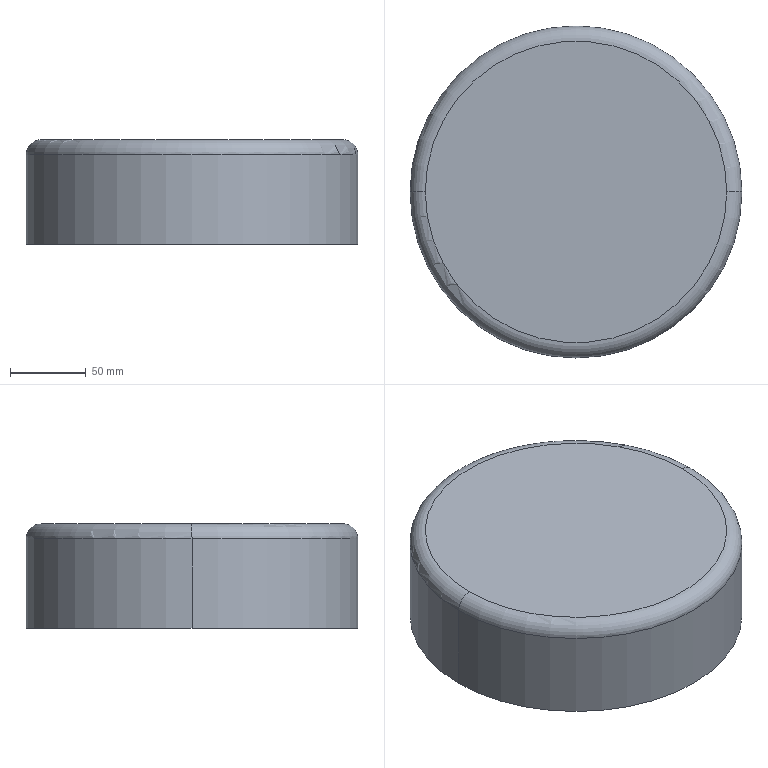Part | SolidWorks | features Fillet 2, Extrusion 1, Shell 1 | 1 solid | 11 faces | box 219 x 219 x 69 mm | volume 466703 mm3 | torus 4 | cylinder 4 | plane 3 | commonest cylinder face diameters 207 x2 219 x2
STEP:
#1=CARTESIAN_POINT('',(-103.5,0.,59.));
#2=VERTEX_POINT('',#1);
#3=CARTESIAN_POINT('',(103.5,0.,59.));
#4=VERTEX_POINT('',#3);
#5=CARTESIAN_POINT('',(0.,0.,59.));
#6=DIRECTION('',(0.,0.,1.));
#7=DIRECTION('',(1.,0.,0.));
#8=AXIS2_PLACEMENT_3D('',#5,#6,#7);
#9=CIRCLE('',#8,103.5);
#10=EDGE_CURVE('',#2,#4,#9,.T.);
#11=ORIENTED_EDGE('',*,*,#10,.F.);
#12=CARTESIAN_POINT('',(-99.5,0.,63.));
#13=VERTEX_POINT('',#12);
#14=CARTESIAN_POINT('',(-99.5,0.,59.));
#15=DIRECTION('',(0.,1.,0.));
#16=DIRECTION('',(-1.,0.,0.));
#17=AXIS2_PLACEMENT_3D('',#14,#15,#16);
#18=CIRCLE('',#17,4.);
#19=EDGE_CURVE('',#2,#13,#18,.T.);
#20=ORIENTED_EDGE('',*,*,#19,.T.);
#21=CARTESIAN_POINT('',(99.5,0.,63.));
#22=VERTEX_POINT('',#21);
#23=CARTESIAN_POINT('',(0.,0.,63.));
#24=DIRECTION('',(0.,0.,-1.));
#25=DIRECTION('',(1.,0.,0.));
#26=AXIS2_PLACEMENT_3D('',#23,#24,#25);
#27=CIRCLE('',#26,99.5);
#28=EDGE_CURVE('',#22,#13,#27,.T.);
#29=ORIENTED_EDGE('',*,*,#28,.F.);
#30=CARTESIAN_POINT('',(99.5,0.,59.));
#31=DIRECTION('',(0.,-1.,0.));
#32=DIRECTION('',(0.,0.,-1.));
#33=AXIS2_PLACEMENT_3D('',#30,#31,#32);
#34=CIRCLE('',#33,4.);
#35=EDGE_CURVE('',#4,#22,#34,.T.);
#36=ORIENTED_EDGE('',*,*,#35,.F.);
#37=EDGE_LOOP('',(#11,#20,#29,#36));
#38=FACE_OUTER_BOUND('',#37,.T.);
#39=CARTESIAN_POINT('',(0.,0.,59.));
#40=DIRECTION('',(0.,0.,1.));
#41=DIRECTION('',(1.,0.,0.));
#42=AXIS2_PLACEMENT_3D('',#39,#40,#41);
#43=TOROIDAL_SURFACE('',#42,99.5,4.);
#44=ADVANCED_FACE('',(#38),#43,.F.);
#45=CARTESIAN_POINT('',(-109.5,0.,59.));
#46=VERTEX_POINT('',#45);
#47=CARTESIAN_POINT('',(109.5,0.,59.));
#48=VERTEX_POINT('',#47);
#49=CARTESIAN_POINT('',(0.,0.,59.));
#50=DIRECTION('',(0.,0.,-1.));
#51=DIRECTION('',(1.,0.,0.));
#52=AXIS2_PLACEMENT_3D('',#49,#50,#51);
#53=CIRCLE('',#52,109.5);
#54=EDGE_CURVE('',#46,#48,#53,.T.);
#55=ORIENTED_EDGE('',*,*,#54,.F.);
#56=CARTESIAN_POINT('',(-99.5,0.,69.));
#57=VERTEX_POINT('',#56);
#58=CARTESIAN_POINT('',(-99.5,0.,59.));
#59=DIRECTION('',(0.,1.,0.));
#60=DIRECTION('',(-1.,0.,0.));
#61=AXIS2_PLACEMENT_3D('',#58,#59,#60);
#62=CIRCLE('',#61,10.);
#63=EDGE_CURVE('',#46,#57,#62,.T.);
#64=ORIENTED_EDGE('',*,*,#63,.T.);
#65=CARTESIAN_POINT('',(99.5,0.,69.));
#66=VERTEX_POINT('',#65);
#67=CARTESIAN_POINT('',(0.,0.,69.));
#68=DIRECTION('',(0.,0.,1.));
#69=DIRECTION('',(1.,0.,0.));
#70=AXIS2_PLACEMENT_3D('',#67,#68,#69);
#71=CIRCLE('',#70,99.5);
#72=EDGE_CURVE('',#66,#57,#71,.T.);
#73=ORIENTED_EDGE('',*,*,#72,.F.);
#74=CARTESIAN_POINT('',(99.5,0.,59.));
#75=DIRECTION('',(0.,-1.,0.));
#76=DIRECTION('',(0.,0.,-1.));
#77=AXIS2_PLACEMENT_3D('',#74,#75,#76);
#78=CIRCLE('',#77,10.);
#79=EDGE_CURVE('',#48,#66,#78,.T.);
#80=ORIENTED_EDGE('',*,*,#79,.F.);
#81=EDGE_LOOP('',(#55,#64,#73,#80));
#82=FACE_OUTER_BOUND('',#81,.T.);
#83=CARTESIAN_POINT('',(0.,0.,59.));
#84=DIRECTION('',(0.,0.,1.));
#85=DIRECTION('',(1.,0.,0.));
#86=AXIS2_PLACEMENT_3D('',#83,#84,#85);
#87=TOROIDAL_SURFACE('',#86,99.5,10.);
#88=ADVANCED_FACE('',(#82),#87,.T.);
#89=ORIENTED_EDGE('',*,*,#10,.T.);
#90=CARTESIAN_POINT('',(103.5,0.,0.));
#91=VERTEX_POINT('',#90);
#92=CARTESIAN_POINT('',(103.5,0.,69.));
#93=DIRECTION('',(0.,0.,-1.));
#94=VECTOR('',#93,1000.);
#95=LINE('',#92,#94);
#96=EDGE_CURVE('',#4,#91,#95,.T.);
#97=ORIENTED_EDGE('',*,*,#96,.T.);
#98=CARTESIAN_POINT('',(-103.5,0.,0.));
#99=VERTEX_POINT('',#98);
#100=CARTESIAN_POINT('',(0.,0.,0.));
#101=DIRECTION('',(0.,0.,1.));
#102=DIRECTION('',(1.,0.,0.));
#103=AXIS2_PLACEMENT_3D('',#100,#101,#102);
#104=CIRCLE('',#103,103.5);
#105=EDGE_CURVE('',#99,#91,#104,.T.);
#106=ORIENTED_EDGE('',*,*,#105,.F.);
#107=CARTESIAN_POINT('',(-103.5,0.,69.));
#108=DIRECTION('',(0.,0.,-1.));
#109=VECTOR('',#108,1000.);
#110=LINE('',#107,#109);
#111=EDGE_CURVE('',#2,#99,#110,.T.);
#112=ORIENTED_EDGE('',*,*,#111,.F.);
#113=EDGE_LOOP('',(#89,#97,#106,#112));
#114=FACE_OUTER_BOUND('',#113,.T.);
#115=CARTESIAN_POINT('',(0.,0.,69.));
#116=DIRECTION('',(0.,0.,-1.));
#117=DIRECTION('',(-1.,0.,0.));
#118=AXIS2_PLACEMENT_3D('',#115,#116,#117);
#119=CYLINDRICAL_SURFACE('',#118,103.5);
#120=ADVANCED_FACE('',(#114),#119,.F.);
#121=ORIENTED_EDGE('',*,*,#54,.T.);
#122=CARTESIAN_POINT('',(109.5,0.,0.));
#123=VERTEX_POINT('',#122);
#124=CARTESIAN_POINT('',(109.5,0.,69.));
#125=DIRECTION('',(0.,0.,-1.));
#126=VECTOR('',#125,1000.);
#127=LINE('',#124,#126);
#128=EDGE_CURVE('',#48,#123,#127,.T.);
#129=ORIENTED_EDGE('',*,*,#128,.T.);
#130=CARTESIAN_POINT('',(-109.5,0.,0.));
#131=VERTEX_POINT('',#130);
#132=CARTESIAN_POINT('',(0.,0.,0.));
#133=DIRECTION('',(0.,0.,1.));
#134=DIRECTION('',(1.,0.,0.));
#135=AXIS2_PLACEMENT_3D('',#132,#133,#134);
#136=CIRCLE('',#135,109.5);
#137=EDGE_CURVE('',#123,#131,#136,.T.);
#138=ORIENTED_EDGE('',*,*,#137,.T.);
#139=CARTESIAN_POINT('',(-109.5,0.,69.));
#140=DIRECTION('',(0.,0.,-1.));
#141=VECTOR('',#140,1000.);
#142=LINE('',#139,#141);
#143=EDGE_CURVE('',#46,#131,#142,.T.);
#144=ORIENTED_EDGE('',*,*,#143,.F.);
#145=EDGE_LOOP('',(#121,#129,#138,#144));
#146=FACE_OUTER_BOUND('',#145,.T.);
#147=CARTESIAN_POINT('',(0.,0.,69.));
#148=DIRECTION('',(0.,0.,-1.));
#149=DIRECTION('',(-1.,0.,0.));
#150=AXIS2_PLACEMENT_3D('',#147,#148,#149);
#151=CYLINDRICAL_SURFACE('',#150,109.5);
#152=ADVANCED_FACE('',(#146),#151,.T.);
#153=ORIENTED_EDGE('',*,*,#128,.F.);
#154=CARTESIAN_POINT('',(0.,0.,59.));
#155=DIRECTION('',(0.,0.,-1.));
#156=DIRECTION('',(1.,0.,0.));
#157=AXIS2_PLACEMENT_3D('',#154,#155,#156);
#158=CIRCLE('',#157,109.5);
#159=EDGE_CURVE('',#48,#46,#158,.T.);
#160=ORIENTED_EDGE('',*,*,#159,.T.);
#161=ORIENTED_EDGE('',*,*,#143,.T.);
#162=CARTESIAN_POINT('',(0.,0.,0.));
#163=DIRECTION('',(0.,0.,1.));
#164=DIRECTION('',(1.,0.,0.));
#165=AXIS2_PLACEMENT_3D('',#162,#163,#164);
#166=CIRCLE('',#165,109.5);
#167=EDGE_CURVE('',#131,#123,#166,.T.);
#168=ORIENTED_EDGE('',*,*,#167,.T.);
#169=EDGE_LOOP('',(#153,#160,#161,#168));
#170=FACE_OUTER_BOUND('',#169,.T.);
#171=CARTESIAN_POINT('',(0.,0.,69.));
#172=DIRECTION('',(0.,0.,-1.));
#173=DIRECTION('',(-1.,0.,0.));
#174=AXIS2_PLACEMENT_3D('',#171,#172,#173);
#175=CYLINDRICAL_SURFACE('',#174,109.5);
#176=ADVANCED_FACE('',(#170),#175,.T.);
#177=ORIENTED_EDGE('',*,*,#72,.T.);
#178=CARTESIAN_POINT('',(0.,0.,69.));
#179=DIRECTION('',(0.,0.,1.));
#180=DIRECTION('',(1.,0.,0.));
#181=AXIS2_PLACEMENT_3D('',#178,#179,#180);
#182=CIRCLE('',#181,99.5);
#183=EDGE_CURVE('',#57,#66,#182,.T.);
#184=ORIENTED_EDGE('',*,*,#183,.T.);
#185=EDGE_LOOP('',(#177,#184));
#186=FACE_OUTER_BOUND('',#185,.T.);
#187=CARTESIAN_POINT('',(0.,0.,69.));
#188=DIRECTION('',(0.,0.,1.));
#189=DIRECTION('',(1.,0.,0.));
#190=AXIS2_PLACEMENT_3D('',#187,#188,#189);
#191=PLANE('',#190);
#192=ADVANCED_FACE('',(#186),#191,.T.);
#193=ORIENTED_EDGE('',*,*,#105,.T.);
#194=CARTESIAN_POINT('',(0.,0.,0.));
#195=DIRECTION('',(0.,0.,1.));
#196=DIRECTION('',(1.,0.,0.));
#197=AXIS2_PLACEMENT_3D('',#194,#195,#196);
#198=CIRCLE('',#197,103.5);
#199=EDGE_CURVE('',#91,#99,#198,.T.);
#200=ORIENTED_EDGE('',*,*,#199,.T.);
#201=EDGE_LOOP('',(#193,#200));
#202=FACE_BOUND('',#201,.T.);
#203=ORIENTED_EDGE('',*,*,#167,.F.);
#204=ORIENTED_EDGE('',*,*,#137,.F.);
#205=EDGE_LOOP('',(#203,#204));
#206=FACE_OUTER_BOUND('',#205,.T.);
#207=CARTESIAN_POINT('',(0.,0.,0.));
#208=DIRECTION('',(0.,0.,1.));
#209=DIRECTION('',(1.,0.,0.));
#210=AXIS2_PLACEMENT_3D('',#207,#208,#209);
#211=PLANE('',#210);
#212=ADVANCED_FACE('',(#202,#206),#211,.F.);
#213=ORIENTED_EDGE('',*,*,#96,.F.);
#214=CARTESIAN_POINT('',(0.,0.,59.));
#215=DIRECTION('',(0.,0.,1.));
#216=DIRECTION('',(1.,0.,0.));
#217=AXIS2_PLACEMENT_3D('',#214,#215,#216);
#218=CIRCLE('',#217,103.5);
#219=EDGE_CURVE('',#4,#2,#218,.T.);
#220=ORIENTED_EDGE('',*,*,#219,.T.);
#221=ORIENTED_EDGE('',*,*,#111,.T.);
#222=ORIENTED_EDGE('',*,*,#199,.F.);
#223=EDGE_LOOP('',(#213,#220,#221,#222));
#224=FACE_OUTER_BOUND('',#223,.T.);
#225=CARTESIAN_POINT('',(0.,0.,69.));
#226=DIRECTION('',(0.,0.,-1.));
#227=DIRECTION('',(-1.,0.,0.));
#228=AXIS2_PLACEMENT_3D('',#225,#226,#227);
#229=CYLINDRICAL_SURFACE('',#228,103.5);
#230=ADVANCED_FACE('',(#224),#229,.F.);
#231=ORIENTED_EDGE('',*,*,#28,.T.);
#232=CARTESIAN_POINT('',(0.,0.,63.));
#233=DIRECTION('',(0.,0.,-1.));
#234=DIRECTION('',(1.,0.,0.));
#235=AXIS2_PLACEMENT_3D('',#232,#233,#234);
#236=CIRCLE('',#235,99.5);
#237=EDGE_CURVE('',#13,#22,#236,.T.);
#238=ORIENTED_EDGE('',*,*,#237,.T.);
#239=EDGE_LOOP('',(#231,#238));
#240=FACE_OUTER_BOUND('',#239,.T.);
#241=CARTESIAN_POINT('',(0.,0.,63.));
#242=DIRECTION('',(0.,0.,1.));
#243=DIRECTION('',(1.,0.,0.));
#244=AXIS2_PLACEMENT_3D('',#241,#242,#243);
#245=PLANE('',#244);
#246=ADVANCED_FACE('',(#240),#245,.F.);
#247=ORIENTED_EDGE('',*,*,#63,.F.);
#248=ORIENTED_EDGE('',*,*,#159,.F.);
#249=ORIENTED_EDGE('',*,*,#79,.T.);
#250=ORIENTED_EDGE('',*,*,#183,.F.);
#251=EDGE_LOOP('',(#247,#248,#249,#250));
#252=FACE_OUTER_BOUND('',#251,.T.);
#253=CARTESIAN_POINT('',(0.,0.,59.));
#254=DIRECTION('',(0.,0.,1.));
#255=DIRECTION('',(1.,0.,0.));
#256=AXIS2_PLACEMENT_3D('',#253,#254,#255);
#257=TOROIDAL_SURFACE('',#256,99.5,10.);
#258=ADVANCED_FACE('',(#252),#257,.T.);
#259=ORIENTED_EDGE('',*,*,#19,.F.);
#260=ORIENTED_EDGE('',*,*,#219,.F.);
#261=ORIENTED_EDGE('',*,*,#35,.T.);
#262=ORIENTED_EDGE('',*,*,#237,.F.);
#263=EDGE_LOOP('',(#259,#260,#261,#262));
#264=FACE_OUTER_BOUND('',#263,.T.);
#265=CARTESIAN_POINT('',(0.,0.,59.));
#266=DIRECTION('',(0.,0.,1.));
#267=DIRECTION('',(1.,0.,0.));
#268=AXIS2_PLACEMENT_3D('',#265,#266,#267);
#269=TOROIDAL_SURFACE('',#268,99.5,4.);
#270=ADVANCED_FACE('',(#264),#269,.F.);
#271=CLOSED_SHELL('',(#44,#88,#120,#152,#176,#192,#212,#230,#246,#258,#270));
#272=MANIFOLD_SOLID_BREP('',#271);
#273=CARTESIAN_POINT('',(0.,0.,0.));
#274=DIRECTION('',(0.,0.,1.));
#275=DIRECTION('',(1.,0.,0.));
#276=AXIS2_PLACEMENT_3D('',#273,#274,#275);
#277=(LENGTH_UNIT()NAMED_UNIT(*)SI_UNIT(.MILLI.,.METRE.));
#278=UNCERTAINTY_MEASURE_WITH_UNIT(LENGTH_MEASURE(0.00001),#277,'','');
#279=(NAMED_UNIT(*)PLANE_ANGLE_UNIT()SI_UNIT($,.RADIAN.));
#280=(NAMED_UNIT(*)SI_UNIT($,.STERADIAN.)SOLID_ANGLE_UNIT());
#281=(GEOMETRIC_REPRESENTATION_CONTEXT(3)GLOBAL_UNCERTAINTY_ASSIGNED_CONTEXT((#278))GLOBAL_UNIT_ASSIGNED_CONTEXT((#277,#279,#280))REPRESENTATION_CONTEXT('',''));
#282=ADVANCED_BREP_SHAPE_REPRESENTATION('',(#272,#276),#281);